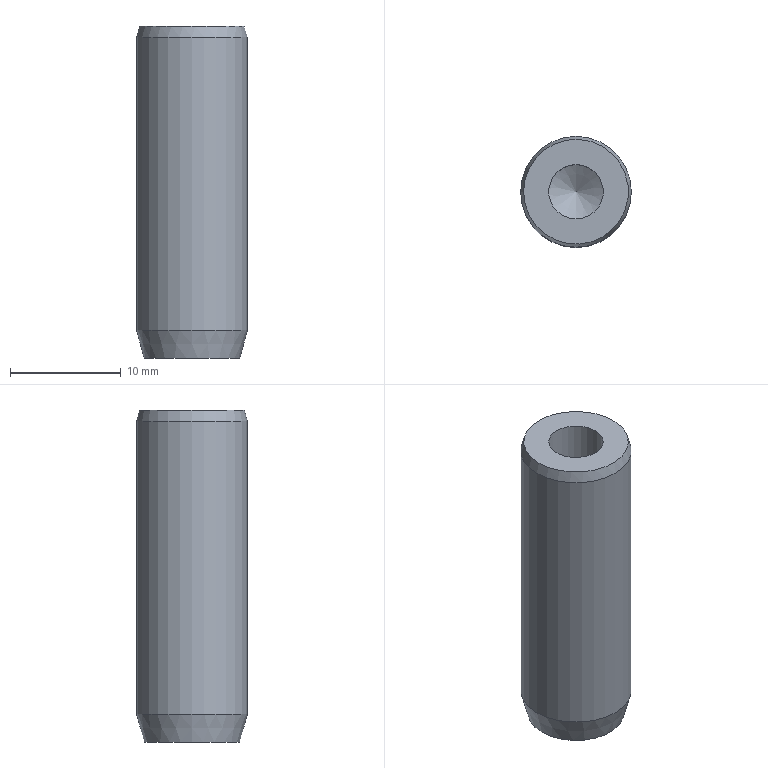Part | NX | features 5003_339_MSHT10-30 2 | 1 solid | 7 faces | box 10 x 10 x 30 mm | volume 2128 mm3 | cone 3 | plane 2 | cylinder 2 | commonest cylinder face diameters 4.917 x1 10 x1
STEP:
#1=CARTESIAN_POINT('',(273.525,-34.541,-172.));
#2=VERTEX_POINT('',#1);
#3=CARTESIAN_POINT('',(273.525,-37.,-172.));
#4=DIRECTION('',(0.,0.,1.));
#5=DIRECTION('',(0.,1.,0.));
#6=AXIS2_PLACEMENT_3D('',#3,#4,#5);
#7=CIRCLE('',#6,2.458);
#8=EDGE_CURVE('',#2,#2,#7,.T.);
#9=ORIENTED_EDGE('',*,*,#8,.F.);
#10=EDGE_LOOP('',(#9));
#11=FACE_BOUND('',#10,.T.);
#12=CARTESIAN_POINT('',(268.793,-37.,-172.));
#13=VERTEX_POINT('',#12);
#14=CARTESIAN_POINT('',(273.525,-37.,-172.));
#15=DIRECTION('',(0.,0.,-1.));
#16=DIRECTION('',(-1.,0.,0.));
#17=AXIS2_PLACEMENT_3D('',#14,#15,#16);
#18=CIRCLE('',#17,4.732);
#19=EDGE_CURVE('',#13,#13,#18,.T.);
#20=ORIENTED_EDGE('',*,*,#19,.F.);
#21=EDGE_LOOP('',(#20));
#22=FACE_BOUND('',#21,.T.);
#23=CARTESIAN_POINT('',(273.525,-37.,-172.));
#24=DIRECTION('',(0.,0.,1.));
#25=DIRECTION('',(1.,0.,0.));
#26=AXIS2_PLACEMENT_3D('',#23,#24,#25);
#27=PLANE('',#26);
#28=ADVANCED_FACE('',(#11,#22),#27,.T.);
#29=ORIENTED_EDGE('',*,*,#19,.T.);
#30=EDGE_LOOP('',(#29));
#31=FACE_BOUND('',#30,.T.);
#32=CARTESIAN_POINT('',(268.525,-37.,-173.));
#33=VERTEX_POINT('',#32);
#34=CARTESIAN_POINT('',(273.525,-37.,-173.));
#35=DIRECTION('',(0.,0.,-1.));
#36=DIRECTION('',(-1.,0.,0.));
#37=AXIS2_PLACEMENT_3D('',#34,#35,#36);
#38=CIRCLE('',#37,5.);
#39=EDGE_CURVE('',#33,#33,#38,.T.);
#40=ORIENTED_EDGE('',*,*,#39,.F.);
#41=EDGE_LOOP('',(#40));
#42=FACE_BOUND('',#41,.T.);
#43=CARTESIAN_POINT('',(273.525,-37.,-173.));
#44=DIRECTION('',(0.,0.,-1.));
#45=DIRECTION('',(-1.,0.,0.));
#46=AXIS2_PLACEMENT_3D('',#43,#44,#45);
#47=CONICAL_SURFACE('',#46,5.,0.2618);
#48=ADVANCED_FACE('',(#31,#42),#47,.T.);
#49=ORIENTED_EDGE('',*,*,#39,.T.);
#50=EDGE_LOOP('',(#49));
#51=FACE_BOUND('',#50,.T.);
#52=CARTESIAN_POINT('',(268.525,-37.,-199.5));
#53=VERTEX_POINT('',#52);
#54=CARTESIAN_POINT('',(273.525,-37.,-199.5));
#55=DIRECTION('',(0.,0.,-1.));
#56=DIRECTION('',(-1.,0.,0.));
#57=AXIS2_PLACEMENT_3D('',#54,#55,#56);
#58=CIRCLE('',#57,5.);
#59=EDGE_CURVE('',#53,#53,#58,.T.);
#60=ORIENTED_EDGE('',*,*,#59,.F.);
#61=EDGE_LOOP('',(#60));
#62=FACE_BOUND('',#61,.T.);
#63=CARTESIAN_POINT('',(273.525,-37.,-202.));
#64=DIRECTION('',(0.,0.,-1.));
#65=DIRECTION('',(-1.,0.,0.));
#66=AXIS2_PLACEMENT_3D('',#63,#64,#65);
#67=CYLINDRICAL_SURFACE('',#66,5.);
#68=ADVANCED_FACE('',(#51,#62),#67,.T.);
#69=ORIENTED_EDGE('',*,*,#59,.T.);
#70=EDGE_LOOP('',(#69));
#71=FACE_BOUND('',#70,.T.);
#72=CARTESIAN_POINT('',(269.195,-37.,-202.));
#73=VERTEX_POINT('',#72);
#74=CARTESIAN_POINT('',(273.525,-37.,-202.));
#75=DIRECTION('',(0.,0.,-1.));
#76=DIRECTION('',(-1.,0.,0.));
#77=AXIS2_PLACEMENT_3D('',#74,#75,#76);
#78=CIRCLE('',#77,4.33);
#79=EDGE_CURVE('',#73,#73,#78,.T.);
#80=ORIENTED_EDGE('',*,*,#79,.F.);
#81=EDGE_LOOP('',(#80));
#82=FACE_BOUND('',#81,.T.);
#83=CARTESIAN_POINT('',(273.525,-37.,-202.));
#84=DIRECTION('',(0.,0.,1.));
#85=DIRECTION('',(1.,0.,0.));
#86=AXIS2_PLACEMENT_3D('',#83,#84,#85);
#87=CONICAL_SURFACE('',#86,4.33,0.2618);
#88=ADVANCED_FACE('',(#71,#82),#87,.T.);
#89=ORIENTED_EDGE('',*,*,#79,.T.);
#90=EDGE_LOOP('',(#89));
#91=FACE_BOUND('',#90,.T.);
#92=CARTESIAN_POINT('',(273.525,-37.,-202.));
#93=DIRECTION('',(0.,0.,-1.));
#94=DIRECTION('',(-1.,0.,0.));
#95=AXIS2_PLACEMENT_3D('',#92,#93,#94);
#96=PLANE('',#95);
#97=ADVANCED_FACE('',(#91),#96,.T.);
#98=CARTESIAN_POINT('',(273.525,-37.,-183.477));
#99=VERTEX_POINT('',#98);
#100=VERTEX_LOOP('',#99);
#101=FACE_BOUND('',#100,.T.);
#102=CARTESIAN_POINT('',(273.525,-34.541,-182.));
#103=VERTEX_POINT('',#102);
#104=CARTESIAN_POINT('',(273.525,-37.,-182.));
#105=DIRECTION('',(0.,0.,1.));
#106=DIRECTION('',(0.,1.,0.));
#107=AXIS2_PLACEMENT_3D('',#104,#105,#106);
#108=CIRCLE('',#107,2.458);
#109=EDGE_CURVE('',#103,#103,#108,.T.);
#110=ORIENTED_EDGE('',*,*,#109,.T.);
#111=EDGE_LOOP('',(#110));
#112=FACE_BOUND('',#111,.T.);
#113=CARTESIAN_POINT('',(273.525,-37.,-182.));
#114=DIRECTION('',(0.,0.,1.));
#115=DIRECTION('',(0.,1.,0.));
#116=AXIS2_PLACEMENT_3D('',#113,#114,#115);
#117=CONICAL_SURFACE('',#116,2.458,1.03);
#118=ADVANCED_FACE('',(#101,#112),#117,.F.);
#119=ORIENTED_EDGE('',*,*,#109,.F.);
#120=EDGE_LOOP('',(#119));
#121=FACE_BOUND('',#120,.T.);
#122=ORIENTED_EDGE('',*,*,#8,.T.);
#123=EDGE_LOOP('',(#122));
#124=FACE_BOUND('',#123,.T.);
#125=CARTESIAN_POINT('',(273.525,-37.,-172.));
#126=DIRECTION('',(0.,0.,1.));
#127=DIRECTION('',(0.,1.,0.));
#128=AXIS2_PLACEMENT_3D('',#125,#126,#127);
#129=CYLINDRICAL_SURFACE('',#128,2.458);
#130=ADVANCED_FACE('',(#121,#124),#129,.F.);
#131=CLOSED_SHELL('',(#28,#48,#68,#88,#97,#118,#130));
#132=MANIFOLD_SOLID_BREP('',#131);
#133=(LENGTH_UNIT()NAMED_UNIT(*)SI_UNIT(.MILLI.,.METRE.));
#134=UNCERTAINTY_MEASURE_WITH_UNIT(LENGTH_MEASURE(0.00001),#133,'','');
#135=(NAMED_UNIT(*)PLANE_ANGLE_UNIT()SI_UNIT($,.RADIAN.));
#136=(NAMED_UNIT(*)SI_UNIT($,.STERADIAN.)SOLID_ANGLE_UNIT());
#137=(GEOMETRIC_REPRESENTATION_CONTEXT(3)GLOBAL_UNCERTAINTY_ASSIGNED_CONTEXT((#134))GLOBAL_UNIT_ASSIGNED_CONTEXT((#133,#135,#136))REPRESENTATION_CONTEXT('',''));
#138=ADVANCED_BREP_SHAPE_REPRESENTATION('',(#132),#137);